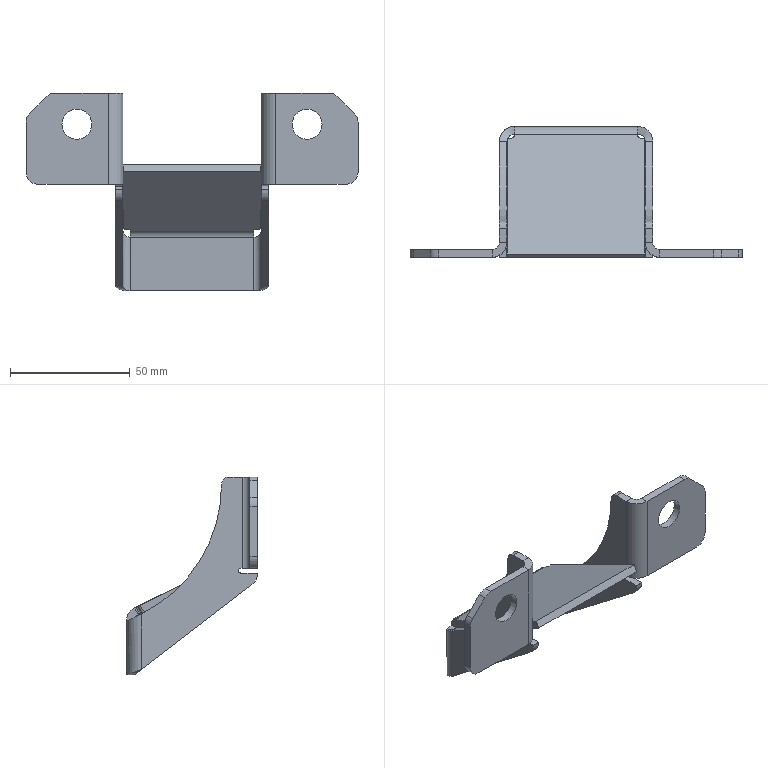Part | SolidWorks | features Fillet 3, ICE 3, EdgeFlange 2, Chamfer 1, FlatPattern 1, SMBaseFlange 1, SheetMetal 1 | 1 solid | 83 faces | box 138.4 x 54.6 x 82.5 mm | volume 33246 mm3 | plane 46 | cylinder 33 | spline 4 | commonest cylinder face diameters 2 x7 6 x7 10 x6 12.4 x5 12.5 x4 12 x2